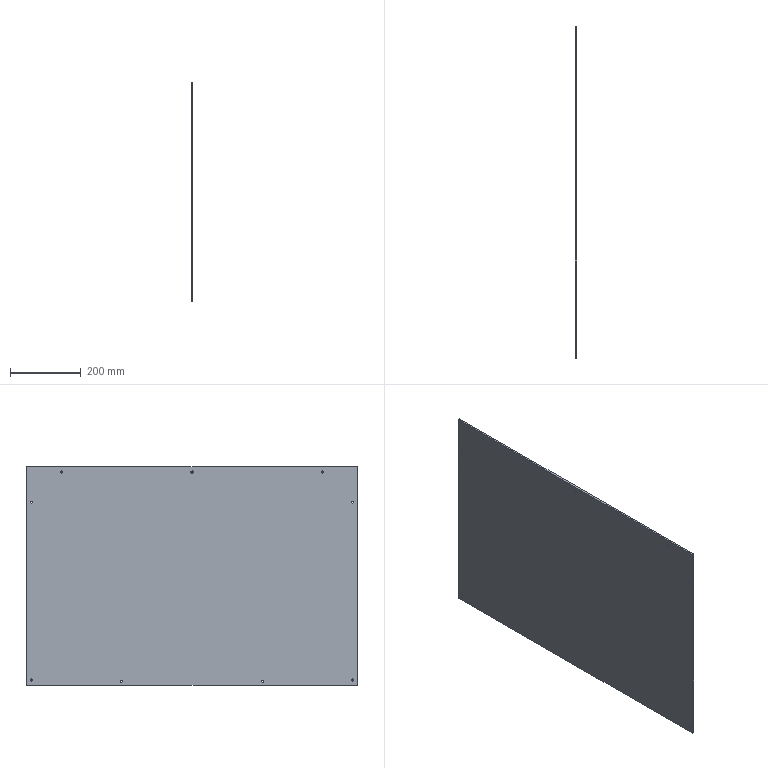Part | SolidWorks | features Chamfer 1, Extrusion 1, ICE 1 | 1 solid | 28 faces | box 5 x 938 x 618 mm | volume 2897138 mm3 | cylinder 18 | plane 10 | commonest cylinder face diameters 6 x18
STEP:
#1=CARTESIAN_POINT('',(5.,-200.,-301.));
#2=VERTEX_POINT('',#1);
#3=CARTESIAN_POINT('',(5.,-200.,-295.));
#4=VERTEX_POINT('',#3);
#5=CARTESIAN_POINT('',(5.,-200.,-298.));
#6=DIRECTION('',(-1.,0.,0.));
#7=DIRECTION('',(0.,0.,1.));
#8=AXIS2_PLACEMENT_3D('',#5,#6,#7);
#9=CIRCLE('',#8,3.);
#10=EDGE_CURVE('',#2,#4,#9,.T.);
#11=ORIENTED_EDGE('',*,*,#10,.F.);
#12=CARTESIAN_POINT('',(0.,-200.,-301.));
#13=VERTEX_POINT('',#12);
#14=CARTESIAN_POINT('',(5.,-200.,-301.));
#15=DIRECTION('',(-1.,0.,0.));
#16=VECTOR('',#15,1000.);
#17=LINE('',#14,#16);
#18=EDGE_CURVE('',#2,#13,#17,.T.);
#19=ORIENTED_EDGE('',*,*,#18,.T.);
#20=CARTESIAN_POINT('',(0.,-200.,-295.));
#21=VERTEX_POINT('',#20);
#22=CARTESIAN_POINT('',(0.,-200.,-298.));
#23=DIRECTION('',(-1.,0.,0.));
#24=DIRECTION('',(0.,0.,1.));
#25=AXIS2_PLACEMENT_3D('',#22,#23,#24);
#26=CIRCLE('',#25,3.);
#27=EDGE_CURVE('',#13,#21,#26,.T.);
#28=ORIENTED_EDGE('',*,*,#27,.T.);
#29=CARTESIAN_POINT('',(5.,-200.,-295.));
#30=DIRECTION('',(-1.,0.,0.));
#31=VECTOR('',#30,1000.);
#32=LINE('',#29,#31);
#33=EDGE_CURVE('',#4,#21,#32,.T.);
#34=ORIENTED_EDGE('',*,*,#33,.F.);
#35=EDGE_LOOP('',(#11,#19,#28,#34));
#36=FACE_OUTER_BOUND('',#35,.T.);
#37=CARTESIAN_POINT('',(5.,-200.,-298.));
#38=DIRECTION('',(-1.,0.,0.));
#39=DIRECTION('',(0.,0.,1.));
#40=AXIS2_PLACEMENT_3D('',#37,#38,#39);
#41=CYLINDRICAL_SURFACE('',#40,3.);
#42=ADVANCED_FACE('',(#36),#41,.F.);
#43=CARTESIAN_POINT('',(5.,200.,-301.));
#44=VERTEX_POINT('',#43);
#45=CARTESIAN_POINT('',(5.,200.,-295.));
#46=VERTEX_POINT('',#45);
#47=CARTESIAN_POINT('',(5.,200.,-298.));
#48=DIRECTION('',(-1.,0.,0.));
#49=DIRECTION('',(0.,0.,1.));
#50=AXIS2_PLACEMENT_3D('',#47,#48,#49);
#51=CIRCLE('',#50,3.);
#52=EDGE_CURVE('',#44,#46,#51,.T.);
#53=ORIENTED_EDGE('',*,*,#52,.F.);
#54=CARTESIAN_POINT('',(0.,200.,-301.));
#55=VERTEX_POINT('',#54);
#56=CARTESIAN_POINT('',(5.,200.,-301.));
#57=DIRECTION('',(-1.,0.,0.));
#58=VECTOR('',#57,1000.);
#59=LINE('',#56,#58);
#60=EDGE_CURVE('',#44,#55,#59,.T.);
#61=ORIENTED_EDGE('',*,*,#60,.T.);
#62=CARTESIAN_POINT('',(0.,200.,-295.));
#63=VERTEX_POINT('',#62);
#64=CARTESIAN_POINT('',(0.,200.,-298.));
#65=DIRECTION('',(-1.,0.,0.));
#66=DIRECTION('',(0.,0.,1.));
#67=AXIS2_PLACEMENT_3D('',#64,#65,#66);
#68=CIRCLE('',#67,3.);
#69=EDGE_CURVE('',#55,#63,#68,.T.);
#70=ORIENTED_EDGE('',*,*,#69,.T.);
#71=CARTESIAN_POINT('',(5.,200.,-295.));
#72=DIRECTION('',(-1.,0.,0.));
#73=VECTOR('',#72,1000.);
#74=LINE('',#71,#73);
#75=EDGE_CURVE('',#46,#63,#74,.T.);
#76=ORIENTED_EDGE('',*,*,#75,.F.);
#77=EDGE_LOOP('',(#53,#61,#70,#76));
#78=FACE_OUTER_BOUND('',#77,.T.);
#79=CARTESIAN_POINT('',(5.,200.,-298.));
#80=DIRECTION('',(-1.,0.,0.));
#81=DIRECTION('',(0.,0.,1.));
#82=AXIS2_PLACEMENT_3D('',#79,#80,#81);
#83=CYLINDRICAL_SURFACE('',#82,3.);
#84=ADVANCED_FACE('',(#78),#83,.F.);
#85=CARTESIAN_POINT('',(5.,0.,291.));
#86=VERTEX_POINT('',#85);
#87=CARTESIAN_POINT('',(5.,0.,297.));
#88=VERTEX_POINT('',#87);
#89=CARTESIAN_POINT('',(5.,0.,294.));
#90=DIRECTION('',(-1.,0.,0.));
#91=DIRECTION('',(0.,0.,1.));
#92=AXIS2_PLACEMENT_3D('',#89,#90,#91);
#93=CIRCLE('',#92,3.);
#94=EDGE_CURVE('',#86,#88,#93,.T.);
#95=ORIENTED_EDGE('',*,*,#94,.F.);
#96=CARTESIAN_POINT('',(0.,0.,291.));
#97=VERTEX_POINT('',#96);
#98=CARTESIAN_POINT('',(5.,0.,291.));
#99=DIRECTION('',(-1.,0.,0.));
#100=VECTOR('',#99,1000.);
#101=LINE('',#98,#100);
#102=EDGE_CURVE('',#86,#97,#101,.T.);
#103=ORIENTED_EDGE('',*,*,#102,.T.);
#104=CARTESIAN_POINT('',(0.,0.,297.));
#105=VERTEX_POINT('',#104);
#106=CARTESIAN_POINT('',(0.,0.,294.));
#107=DIRECTION('',(-1.,0.,0.));
#108=DIRECTION('',(0.,0.,1.));
#109=AXIS2_PLACEMENT_3D('',#106,#107,#108);
#110=CIRCLE('',#109,3.);
#111=EDGE_CURVE('',#97,#105,#110,.T.);
#112=ORIENTED_EDGE('',*,*,#111,.T.);
#113=CARTESIAN_POINT('',(5.,0.,297.));
#114=DIRECTION('',(-1.,0.,0.));
#115=VECTOR('',#114,1000.);
#116=LINE('',#113,#115);
#117=EDGE_CURVE('',#88,#105,#116,.T.);
#118=ORIENTED_EDGE('',*,*,#117,.F.);
#119=EDGE_LOOP('',(#95,#103,#112,#118));
#120=FACE_OUTER_BOUND('',#119,.T.);
#121=CARTESIAN_POINT('',(5.,0.,294.));
#122=DIRECTION('',(-1.,0.,0.));
#123=DIRECTION('',(0.,0.,1.));
#124=AXIS2_PLACEMENT_3D('',#121,#122,#123);
#125=CYLINDRICAL_SURFACE('',#124,3.);
#126=ADVANCED_FACE('',(#120),#125,.F.);
#127=CARTESIAN_POINT('',(5.,-454.,206.));
#128=VERTEX_POINT('',#127);
#129=CARTESIAN_POINT('',(5.,-454.,212.));
#130=VERTEX_POINT('',#129);
#131=CARTESIAN_POINT('',(5.,-454.,209.));
#132=DIRECTION('',(-1.,0.,0.));
#133=DIRECTION('',(0.,0.,1.));
#134=AXIS2_PLACEMENT_3D('',#131,#132,#133);
#135=CIRCLE('',#134,3.);
#136=EDGE_CURVE('',#128,#130,#135,.T.);
#137=ORIENTED_EDGE('',*,*,#136,.F.);
#138=CARTESIAN_POINT('',(0.,-454.,206.));
#139=VERTEX_POINT('',#138);
#140=CARTESIAN_POINT('',(5.,-454.,206.));
#141=DIRECTION('',(-1.,0.,0.));
#142=VECTOR('',#141,1000.);
#143=LINE('',#140,#142);
#144=EDGE_CURVE('',#128,#139,#143,.T.);
#145=ORIENTED_EDGE('',*,*,#144,.T.);
#146=CARTESIAN_POINT('',(0.,-454.,212.));
#147=VERTEX_POINT('',#146);
#148=CARTESIAN_POINT('',(0.,-454.,209.));
#149=DIRECTION('',(-1.,0.,0.));
#150=DIRECTION('',(0.,0.,1.));
#151=AXIS2_PLACEMENT_3D('',#148,#149,#150);
#152=CIRCLE('',#151,3.);
#153=EDGE_CURVE('',#139,#147,#152,.T.);
#154=ORIENTED_EDGE('',*,*,#153,.T.);
#155=CARTESIAN_POINT('',(5.,-454.,212.));
#156=DIRECTION('',(-1.,0.,0.));
#157=VECTOR('',#156,1000.);
#158=LINE('',#155,#157);
#159=EDGE_CURVE('',#130,#147,#158,.T.);
#160=ORIENTED_EDGE('',*,*,#159,.F.);
#161=EDGE_LOOP('',(#137,#145,#154,#160));
#162=FACE_OUTER_BOUND('',#161,.T.);
#163=CARTESIAN_POINT('',(5.,-454.,209.));
#164=DIRECTION('',(-1.,0.,0.));
#165=DIRECTION('',(0.,0.,1.));
#166=AXIS2_PLACEMENT_3D('',#163,#164,#165);
#167=CYLINDRICAL_SURFACE('',#166,3.);
#168=ADVANCED_FACE('',(#162),#167,.F.);
#169=CARTESIAN_POINT('',(5.,-369.,291.));
#170=VERTEX_POINT('',#169);
#171=CARTESIAN_POINT('',(5.,-369.,297.));
#172=VERTEX_POINT('',#171);
#173=CARTESIAN_POINT('',(5.,-369.,294.));
#174=DIRECTION('',(-1.,0.,0.));
#175=DIRECTION('',(0.,0.,1.));
#176=AXIS2_PLACEMENT_3D('',#173,#174,#175);
#177=CIRCLE('',#176,3.);
#178=EDGE_CURVE('',#170,#172,#177,.T.);
#179=ORIENTED_EDGE('',*,*,#178,.F.);
#180=CARTESIAN_POINT('',(0.,-369.,291.));
#181=VERTEX_POINT('',#180);
#182=CARTESIAN_POINT('',(5.,-369.,291.));
#183=DIRECTION('',(-1.,0.,0.));
#184=VECTOR('',#183,1000.);
#185=LINE('',#182,#184);
#186=EDGE_CURVE('',#170,#181,#185,.T.);
#187=ORIENTED_EDGE('',*,*,#186,.T.);
#188=CARTESIAN_POINT('',(0.,-369.,297.));
#189=VERTEX_POINT('',#188);
#190=CARTESIAN_POINT('',(0.,-369.,294.));
#191=DIRECTION('',(-1.,0.,0.));
#192=DIRECTION('',(0.,0.,1.));
#193=AXIS2_PLACEMENT_3D('',#190,#191,#192);
#194=CIRCLE('',#193,3.);
#195=EDGE_CURVE('',#181,#189,#194,.T.);
#196=ORIENTED_EDGE('',*,*,#195,.T.);
#197=CARTESIAN_POINT('',(5.,-369.,297.));
#198=DIRECTION('',(-1.,0.,0.));
#199=VECTOR('',#198,1000.);
#200=LINE('',#197,#199);
#201=EDGE_CURVE('',#172,#189,#200,.T.);
#202=ORIENTED_EDGE('',*,*,#201,.F.);
#203=EDGE_LOOP('',(#179,#187,#196,#202));
#204=FACE_OUTER_BOUND('',#203,.T.);
#205=CARTESIAN_POINT('',(5.,-369.,294.));
#206=DIRECTION('',(-1.,0.,0.));
#207=DIRECTION('',(0.,0.,1.));
#208=AXIS2_PLACEMENT_3D('',#205,#206,#207);
#209=CYLINDRICAL_SURFACE('',#208,3.);
#210=ADVANCED_FACE('',(#204),#209,.F.);
#211=CARTESIAN_POINT('',(5.,369.,291.));
#212=VERTEX_POINT('',#211);
#213=CARTESIAN_POINT('',(5.,369.,297.));
#214=VERTEX_POINT('',#213);
#215=CARTESIAN_POINT('',(5.,369.,294.));
#216=DIRECTION('',(-1.,0.,0.));
#217=DIRECTION('',(0.,0.,1.));
#218=AXIS2_PLACEMENT_3D('',#215,#216,#217);
#219=CIRCLE('',#218,3.);
#220=EDGE_CURVE('',#212,#214,#219,.T.);
#221=ORIENTED_EDGE('',*,*,#220,.F.);
#222=CARTESIAN_POINT('',(0.,369.,291.));
#223=VERTEX_POINT('',#222);
#224=CARTESIAN_POINT('',(5.,369.,291.));
#225=DIRECTION('',(-1.,0.,0.));
#226=VECTOR('',#225,1000.);
#227=LINE('',#224,#226);
#228=EDGE_CURVE('',#212,#223,#227,.T.);
#229=ORIENTED_EDGE('',*,*,#228,.T.);
#230=CARTESIAN_POINT('',(0.,369.,297.));
#231=VERTEX_POINT('',#230);
#232=CARTESIAN_POINT('',(0.,369.,294.));
#233=DIRECTION('',(-1.,0.,0.));
#234=DIRECTION('',(0.,0.,1.));
#235=AXIS2_PLACEMENT_3D('',#232,#233,#234);
#236=CIRCLE('',#235,3.);
#237=EDGE_CURVE('',#223,#231,#236,.T.);
#238=ORIENTED_EDGE('',*,*,#237,.T.);
#239=CARTESIAN_POINT('',(5.,369.,297.));
#240=DIRECTION('',(-1.,0.,0.));
#241=VECTOR('',#240,1000.);
#242=LINE('',#239,#241);
#243=EDGE_CURVE('',#214,#231,#242,.T.);
#244=ORIENTED_EDGE('',*,*,#243,.F.);
#245=EDGE_LOOP('',(#221,#229,#238,#244));
#246=FACE_OUTER_BOUND('',#245,.T.);
#247=CARTESIAN_POINT('',(5.,369.,294.));
#248=DIRECTION('',(-1.,0.,0.));
#249=DIRECTION('',(0.,0.,1.));
#250=AXIS2_PLACEMENT_3D('',#247,#248,#249);
#251=CYLINDRICAL_SURFACE('',#250,3.);
#252=ADVANCED_FACE('',(#246),#251,.F.);
#253=CARTESIAN_POINT('',(5.,454.,206.));
#254=VERTEX_POINT('',#253);
#255=CARTESIAN_POINT('',(5.,454.,212.));
#256=VERTEX_POINT('',#255);
#257=CARTESIAN_POINT('',(5.,454.,209.));
#258=DIRECTION('',(-1.,0.,0.));
#259=DIRECTION('',(0.,0.,1.));
#260=AXIS2_PLACEMENT_3D('',#257,#258,#259);
#261=CIRCLE('',#260,3.);
#262=EDGE_CURVE('',#254,#256,#261,.T.);
#263=ORIENTED_EDGE('',*,*,#262,.F.);
#264=CARTESIAN_POINT('',(0.,454.,206.));
#265=VERTEX_POINT('',#264);
#266=CARTESIAN_POINT('',(5.,454.,206.));
#267=DIRECTION('',(-1.,0.,0.));
#268=VECTOR('',#267,1000.);
#269=LINE('',#266,#268);
#270=EDGE_CURVE('',#254,#265,#269,.T.);
#271=ORIENTED_EDGE('',*,*,#270,.T.);
#272=CARTESIAN_POINT('',(0.,454.,212.));
#273=VERTEX_POINT('',#272);
#274=CARTESIAN_POINT('',(0.,454.,209.));
#275=DIRECTION('',(-1.,0.,0.));
#276=DIRECTION('',(0.,0.,1.));
#277=AXIS2_PLACEMENT_3D('',#274,#275,#276);
#278=CIRCLE('',#277,3.);
#279=EDGE_CURVE('',#265,#273,#278,.T.);
#280=ORIENTED_EDGE('',*,*,#279,.T.);
#281=CARTESIAN_POINT('',(5.,454.,212.));
#282=DIRECTION('',(-1.,0.,0.));
#283=VECTOR('',#282,1000.);
#284=LINE('',#281,#283);
#285=EDGE_CURVE('',#256,#273,#284,.T.);
#286=ORIENTED_EDGE('',*,*,#285,.F.);
#287=EDGE_LOOP('',(#263,#271,#280,#286));
#288=FACE_OUTER_BOUND('',#287,.T.);
#289=CARTESIAN_POINT('',(5.,454.,209.));
#290=DIRECTION('',(-1.,0.,0.));
#291=DIRECTION('',(0.,0.,1.));
#292=AXIS2_PLACEMENT_3D('',#289,#290,#291);
#293=CYLINDRICAL_SURFACE('',#292,3.);
#294=ADVANCED_FACE('',(#288),#293,.F.);
#295=CARTESIAN_POINT('',(5.,-454.,-297.));
#296=VERTEX_POINT('',#295);
#297=CARTESIAN_POINT('',(5.,-454.,-291.));
#298=VERTEX_POINT('',#297);
#299=CARTESIAN_POINT('',(5.,-454.,-294.));
#300=DIRECTION('',(-1.,0.,0.));
#301=DIRECTION('',(0.,0.,-1.));
#302=AXIS2_PLACEMENT_3D('',#299,#300,#301);
#303=CIRCLE('',#302,3.);
#304=EDGE_CURVE('',#296,#298,#303,.T.);
#305=ORIENTED_EDGE('',*,*,#304,.F.);
#306=CARTESIAN_POINT('',(0.,-454.,-297.));
#307=VERTEX_POINT('',#306);
#308=CARTESIAN_POINT('',(5.,-454.,-297.));
#309=DIRECTION('',(-1.,0.,0.));
#310=VECTOR('',#309,1000.);
#311=LINE('',#308,#310);
#312=EDGE_CURVE('',#296,#307,#311,.T.);
#313=ORIENTED_EDGE('',*,*,#312,.T.);
#314=CARTESIAN_POINT('',(0.,-454.,-291.));
#315=VERTEX_POINT('',#314);
#316=CARTESIAN_POINT('',(0.,-454.,-294.));
#317=DIRECTION('',(-1.,0.,0.));
#318=DIRECTION('',(0.,0.,-1.));
#319=AXIS2_PLACEMENT_3D('',#316,#317,#318);
#320=CIRCLE('',#319,3.);
#321=EDGE_CURVE('',#307,#315,#320,.T.);
#322=ORIENTED_EDGE('',*,*,#321,.T.);
#323=CARTESIAN_POINT('',(5.,-454.,-291.));
#324=DIRECTION('',(-1.,0.,0.));
#325=VECTOR('',#324,1000.);
#326=LINE('',#323,#325);
#327=EDGE_CURVE('',#298,#315,#326,.T.);
#328=ORIENTED_EDGE('',*,*,#327,.F.);
#329=EDGE_LOOP('',(#305,#313,#322,#328));
#330=FACE_OUTER_BOUND('',#329,.T.);
#331=CARTESIAN_POINT('',(5.,-454.,-294.));
#332=DIRECTION('',(-1.,0.,0.));
#333=DIRECTION('',(0.,0.,1.));
#334=AXIS2_PLACEMENT_3D('',#331,#332,#333);
#335=CYLINDRICAL_SURFACE('',#334,3.);
#336=ADVANCED_FACE('',(#330),#335,.F.);
#337=CARTESIAN_POINT('',(5.,454.,-297.));
#338=VERTEX_POINT('',#337);
#339=CARTESIAN_POINT('',(5.,454.,-291.));
#340=VERTEX_POINT('',#339);
#341=CARTESIAN_POINT('',(5.,454.,-294.));
#342=DIRECTION('',(-1.,0.,0.));
#343=DIRECTION('',(0.,0.,1.));
#344=AXIS2_PLACEMENT_3D('',#341,#342,#343);
#345=CIRCLE('',#344,3.);
#346=EDGE_CURVE('',#338,#340,#345,.T.);
#347=ORIENTED_EDGE('',*,*,#346,.F.);
#348=CARTESIAN_POINT('',(0.,454.,-297.));
#349=VERTEX_POINT('',#348);
#350=CARTESIAN_POINT('',(5.,454.,-297.));
#351=DIRECTION('',(-1.,0.,0.));
#352=VECTOR('',#351,1000.);
#353=LINE('',#350,#352);
#354=EDGE_CURVE('',#338,#349,#353,.T.);
#355=ORIENTED_EDGE('',*,*,#354,.T.);
#356=CARTESIAN_POINT('',(0.,454.,-291.));
#357=VERTEX_POINT('',#356);
#358=CARTESIAN_POINT('',(0.,454.,-294.));
#359=DIRECTION('',(-1.,0.,0.));
#360=DIRECTION('',(0.,0.,1.));
#361=AXIS2_PLACEMENT_3D('',#358,#359,#360);
#362=CIRCLE('',#361,3.);
#363=EDGE_CURVE('',#349,#357,#362,.T.);
#364=ORIENTED_EDGE('',*,*,#363,.T.);
#365=CARTESIAN_POINT('',(5.,454.,-291.));
#366=DIRECTION('',(-1.,0.,0.));
#367=VECTOR('',#366,1000.);
#368=LINE('',#365,#367);
#369=EDGE_CURVE('',#340,#357,#368,.T.);
#370=ORIENTED_EDGE('',*,*,#369,.F.);
#371=EDGE_LOOP('',(#347,#355,#364,#370));
#372=FACE_OUTER_BOUND('',#371,.T.);
#373=CARTESIAN_POINT('',(5.,454.,-294.));
#374=DIRECTION('',(-1.,0.,0.));
#375=DIRECTION('',(0.,0.,1.));
#376=AXIS2_PLACEMENT_3D('',#373,#374,#375);
#377=CYLINDRICAL_SURFACE('',#376,3.);
#378=ADVANCED_FACE('',(#372),#377,.F.);
#379=CARTESIAN_POINT('',(0.,468.,309.));
#380=VERTEX_POINT('',#379);
#381=CARTESIAN_POINT('',(0.,-468.,309.));
#382=VERTEX_POINT('',#381);
#383=CARTESIAN_POINT('',(0.,469.,309.));
#384=DIRECTION('',(0.,-1.,0.));
#385=VECTOR('',#384,1000.);
#386=LINE('',#383,#385);
#387=EDGE_CURVE('',#380,#382,#386,.T.);
#388=ORIENTED_EDGE('',*,*,#387,.T.);
#389=CARTESIAN_POINT('',(5.,-468.,309.));
#390=VERTEX_POINT('',#389);
#391=CARTESIAN_POINT('',(5.,-468.,309.));
#392=DIRECTION('',(1.,0.,0.));
#393=VECTOR('',#392,1000.);
#394=LINE('',#391,#393);
#395=EDGE_CURVE('',#382,#390,#394,.T.);
#396=ORIENTED_EDGE('',*,*,#395,.T.);
#397=CARTESIAN_POINT('',(5.,468.,309.));
#398=VERTEX_POINT('',#397);
#399=CARTESIAN_POINT('',(5.,469.,309.));
#400=DIRECTION('',(0.,-1.,0.));
#401=VECTOR('',#400,1000.);
#402=LINE('',#399,#401);
#403=EDGE_CURVE('',#398,#390,#402,.T.);
#404=ORIENTED_EDGE('',*,*,#403,.F.);
#405=CARTESIAN_POINT('',(5.,468.,309.));
#406=DIRECTION('',(-1.,0.,0.));
#407=VECTOR('',#406,1000.);
#408=LINE('',#405,#407);
#409=EDGE_CURVE('',#398,#380,#408,.T.);
#410=ORIENTED_EDGE('',*,*,#409,.T.);
#411=EDGE_LOOP('',(#388,#396,#404,#410));
#412=FACE_OUTER_BOUND('',#411,.T.);
#413=CARTESIAN_POINT('',(5.,469.,309.));
#414=DIRECTION('',(0.,0.,-1.));
#415=DIRECTION('',(0.,1.,0.));
#416=AXIS2_PLACEMENT_3D('',#413,#414,#415);
#417=PLANE('',#416);
#418=ADVANCED_FACE('',(#412),#417,.F.);
#419=CARTESIAN_POINT('',(0.,-469.,308.));
#420=VERTEX_POINT('',#419);
#421=CARTESIAN_POINT('',(0.,-469.,-308.));
#422=VERTEX_POINT('',#421);
#423=CARTESIAN_POINT('',(0.,-469.,-309.));
#424=DIRECTION('',(0.,0.,-1.));
#425=VECTOR('',#424,1000.);
#426=LINE('',#423,#425);
#427=EDGE_CURVE('',#420,#422,#426,.T.);
#428=ORIENTED_EDGE('',*,*,#427,.T.);
#429=CARTESIAN_POINT('',(5.,-469.,-308.));
#430=VERTEX_POINT('',#429);
#431=CARTESIAN_POINT('',(5.,-469.,-308.));
#432=DIRECTION('',(1.,0.,0.));
#433=VECTOR('',#432,1000.);
#434=LINE('',#431,#433);
#435=EDGE_CURVE('',#422,#430,#434,.T.);
#436=ORIENTED_EDGE('',*,*,#435,.T.);
#437=CARTESIAN_POINT('',(5.,-469.,308.));
#438=VERTEX_POINT('',#437);
#439=CARTESIAN_POINT('',(5.,-469.,-309.));
#440=DIRECTION('',(0.,0.,-1.));
#441=VECTOR('',#440,1000.);
#442=LINE('',#439,#441);
#443=EDGE_CURVE('',#438,#430,#442,.T.);
#444=ORIENTED_EDGE('',*,*,#443,.F.);
#445=CARTESIAN_POINT('',(5.,-469.,308.));
#446=DIRECTION('',(-1.,0.,0.));
#447=VECTOR('',#446,1000.);
#448=LINE('',#445,#447);
#449=EDGE_CURVE('',#438,#420,#448,.T.);
#450=ORIENTED_EDGE('',*,*,#449,.T.);
#451=EDGE_LOOP('',(#428,#436,#444,#450));
#452=FACE_OUTER_BOUND('',#451,.T.);
#453=CARTESIAN_POINT('',(5.,-469.,-309.));
#454=DIRECTION('',(0.,1.,0.));
#455=DIRECTION('',(0.,0.,1.));
#456=AXIS2_PLACEMENT_3D('',#453,#454,#455);
#457=PLANE('',#456);
#458=ADVANCED_FACE('',(#452),#457,.F.);
#459=CARTESIAN_POINT('',(5.,-468.,-309.));
#460=VERTEX_POINT('',#459);
#461=CARTESIAN_POINT('',(5.,468.,-309.));
#462=VERTEX_POINT('',#461);
#463=CARTESIAN_POINT('',(5.,469.,-309.));
#464=DIRECTION('',(0.,1.,0.));
#465=VECTOR('',#464,1000.);
#466=LINE('',#463,#465);
#467=EDGE_CURVE('',#460,#462,#466,.T.);
#468=ORIENTED_EDGE('',*,*,#467,.F.);
#469=CARTESIAN_POINT('',(0.,-468.,-309.));
#470=VERTEX_POINT('',#469);
#471=CARTESIAN_POINT('',(5.,-468.,-309.));
#472=DIRECTION('',(-1.,0.,0.));
#473=VECTOR('',#472,1000.);
#474=LINE('',#471,#473);
#475=EDGE_CURVE('',#460,#470,#474,.T.);
#476=ORIENTED_EDGE('',*,*,#475,.T.);
#477=CARTESIAN_POINT('',(0.,468.,-309.));
#478=VERTEX_POINT('',#477);
#479=CARTESIAN_POINT('',(0.,469.,-309.));
#480=DIRECTION('',(0.,1.,0.));
#481=VECTOR('',#480,1000.);
#482=LINE('',#479,#481);
#483=EDGE_CURVE('',#470,#478,#482,.T.);
#484=ORIENTED_EDGE('',*,*,#483,.T.);
#485=CARTESIAN_POINT('',(5.,468.,-309.));
#486=DIRECTION('',(1.,0.,0.));
#487=VECTOR('',#486,1000.);
#488=LINE('',#485,#487);
#489=EDGE_CURVE('',#478,#462,#488,.T.);
#490=ORIENTED_EDGE('',*,*,#489,.T.);
#491=EDGE_LOOP('',(#468,#476,#484,#490));
#492=FACE_OUTER_BOUND('',#491,.T.);
#493=CARTESIAN_POINT('',(5.,469.,-309.));
#494=DIRECTION('',(0.,0.,1.));
#495=DIRECTION('',(0.,-1.,0.));
#496=AXIS2_PLACEMENT_3D('',#493,#494,#495);
#497=PLANE('',#496);
#498=ADVANCED_FACE('',(#492),#497,.F.);
#499=CARTESIAN_POINT('',(5.,469.,-308.));
#500=VERTEX_POINT('',#499);
#501=CARTESIAN_POINT('',(5.,469.,308.));
#502=VERTEX_POINT('',#501);
#503=CARTESIAN_POINT('',(5.,469.,-309.));
#504=DIRECTION('',(0.,0.,1.));
#505=VECTOR('',#504,1000.);
#506=LINE('',#503,#505);
#507=EDGE_CURVE('',#500,#502,#506,.T.);
#508=ORIENTED_EDGE('',*,*,#507,.F.);
#509=CARTESIAN_POINT('',(0.,469.,-308.));
#510=VERTEX_POINT('',#509);
#511=CARTESIAN_POINT('',(5.,469.,-308.));
#512=DIRECTION('',(-1.,0.,0.));
#513=VECTOR('',#512,1000.);
#514=LINE('',#511,#513);
#515=EDGE_CURVE('',#500,#510,#514,.T.);
#516=ORIENTED_EDGE('',*,*,#515,.T.);
#517=CARTESIAN_POINT('',(0.,469.,308.));
#518=VERTEX_POINT('',#517);
#519=CARTESIAN_POINT('',(0.,469.,-309.));
#520=DIRECTION('',(0.,0.,1.));
#521=VECTOR('',#520,1000.);
#522=LINE('',#519,#521);
#523=EDGE_CURVE('',#510,#518,#522,.T.);
#524=ORIENTED_EDGE('',*,*,#523,.T.);
#525=CARTESIAN_POINT('',(5.,469.,308.));
#526=DIRECTION('',(1.,0.,0.));
#527=VECTOR('',#526,1000.);
#528=LINE('',#525,#527);
#529=EDGE_CURVE('',#518,#502,#528,.T.);
#530=ORIENTED_EDGE('',*,*,#529,.T.);
#531=EDGE_LOOP('',(#508,#516,#524,#530));
#532=FACE_OUTER_BOUND('',#531,.T.);
#533=CARTESIAN_POINT('',(5.,469.,-309.));
#534=DIRECTION('',(0.,-1.,0.));
#535=DIRECTION('',(0.,0.,-1.));
#536=AXIS2_PLACEMENT_3D('',#533,#534,#535);
#537=PLANE('',#536);
#538=ADVANCED_FACE('',(#532),#537,.F.);
#539=CARTESIAN_POINT('',(5.,-200.,-298.));
#540=DIRECTION('',(-1.,0.,0.));
#541=DIRECTION('',(0.,0.,1.));
#542=AXIS2_PLACEMENT_3D('',#539,#540,#541);
#543=CIRCLE('',#542,3.);
#544=EDGE_CURVE('',#4,#2,#543,.T.);
#545=ORIENTED_EDGE('',*,*,#544,.T.);
#546=ORIENTED_EDGE('',*,*,#10,.T.);
#547=EDGE_LOOP('',(#545,#546));
#548=FACE_BOUND('',#547,.T.);
#549=CARTESIAN_POINT('',(5.,200.,-298.));
#550=DIRECTION('',(-1.,0.,0.));
#551=DIRECTION('',(0.,0.,1.));
#552=AXIS2_PLACEMENT_3D('',#549,#550,#551);
#553=CIRCLE('',#552,3.);
#554=EDGE_CURVE('',#46,#44,#553,.T.);
#555=ORIENTED_EDGE('',*,*,#554,.T.);
#556=ORIENTED_EDGE('',*,*,#52,.T.);
#557=EDGE_LOOP('',(#555,#556));
#558=FACE_BOUND('',#557,.T.);
#559=CARTESIAN_POINT('',(5.,0.,294.));
#560=DIRECTION('',(-1.,0.,0.));
#561=DIRECTION('',(0.,0.,1.));
#562=AXIS2_PLACEMENT_3D('',#559,#560,#561);
#563=CIRCLE('',#562,3.);
#564=EDGE_CURVE('',#88,#86,#563,.T.);
#565=ORIENTED_EDGE('',*,*,#564,.T.);
#566=ORIENTED_EDGE('',*,*,#94,.T.);
#567=EDGE_LOOP('',(#565,#566));
#568=FACE_BOUND('',#567,.T.);
#569=CARTESIAN_POINT('',(5.,-454.,209.));
#570=DIRECTION('',(-1.,0.,0.));
#571=DIRECTION('',(0.,0.,1.));
#572=AXIS2_PLACEMENT_3D('',#569,#570,#571);
#573=CIRCLE('',#572,3.);
#574=EDGE_CURVE('',#130,#128,#573,.T.);
#575=ORIENTED_EDGE('',*,*,#574,.T.);
#576=ORIENTED_EDGE('',*,*,#136,.T.);
#577=EDGE_LOOP('',(#575,#576));
#578=FACE_BOUND('',#577,.T.);
#579=CARTESIAN_POINT('',(5.,-369.,294.));
#580=DIRECTION('',(-1.,0.,0.));
#581=DIRECTION('',(0.,0.,1.));
#582=AXIS2_PLACEMENT_3D('',#579,#580,#581);
#583=CIRCLE('',#582,3.);
#584=EDGE_CURVE('',#172,#170,#583,.T.);
#585=ORIENTED_EDGE('',*,*,#584,.T.);
#586=ORIENTED_EDGE('',*,*,#178,.T.);
#587=EDGE_LOOP('',(#585,#586));
#588=FACE_BOUND('',#587,.T.);
#589=CARTESIAN_POINT('',(5.,369.,294.));
#590=DIRECTION('',(-1.,0.,0.));
#591=DIRECTION('',(0.,0.,1.));
#592=AXIS2_PLACEMENT_3D('',#589,#590,#591);
#593=CIRCLE('',#592,3.);
#594=EDGE_CURVE('',#214,#212,#593,.T.);
#595=ORIENTED_EDGE('',*,*,#594,.T.);
#596=ORIENTED_EDGE('',*,*,#220,.T.);
#597=EDGE_LOOP('',(#595,#596));
#598=FACE_BOUND('',#597,.T.);
#599=CARTESIAN_POINT('',(5.,454.,209.));
#600=DIRECTION('',(-1.,0.,0.));
#601=DIRECTION('',(0.,0.,1.));
#602=AXIS2_PLACEMENT_3D('',#599,#600,#601);
#603=CIRCLE('',#602,3.);
#604=EDGE_CURVE('',#256,#254,#603,.T.);
#605=ORIENTED_EDGE('',*,*,#604,.T.);
#606=ORIENTED_EDGE('',*,*,#262,.T.);
#607=EDGE_LOOP('',(#605,#606));
#608=FACE_BOUND('',#607,.T.);
#609=CARTESIAN_POINT('',(5.,-454.,-294.));
#610=DIRECTION('',(-1.,0.,0.));
#611=DIRECTION('',(0.,0.,-1.));
#612=AXIS2_PLACEMENT_3D('',#609,#610,#611);
#613=CIRCLE('',#612,3.);
#614=EDGE_CURVE('',#298,#296,#613,.T.);
#615=ORIENTED_EDGE('',*,*,#614,.T.);
#616=ORIENTED_EDGE('',*,*,#304,.T.);
#617=EDGE_LOOP('',(#615,#616));
#618=FACE_BOUND('',#617,.T.);
#619=CARTESIAN_POINT('',(5.,454.,-294.));
#620=DIRECTION('',(-1.,0.,0.));
#621=DIRECTION('',(0.,0.,1.));
#622=AXIS2_PLACEMENT_3D('',#619,#620,#621);
#623=CIRCLE('',#622,3.);
#624=EDGE_CURVE('',#340,#338,#623,.T.);
#625=ORIENTED_EDGE('',*,*,#624,.T.);
#626=ORIENTED_EDGE('',*,*,#346,.T.);
#627=EDGE_LOOP('',(#625,#626));
#628=FACE_BOUND('',#627,.T.);
#629=ORIENTED_EDGE('',*,*,#443,.T.);
#630=CARTESIAN_POINT('',(5.,-468.,-309.));
#631=DIRECTION('',(0.,0.7071,-0.7071));
#632=VECTOR('',#631,1000.);
#633=LINE('',#630,#632);
#634=EDGE_CURVE('',#430,#460,#633,.T.);
#635=ORIENTED_EDGE('',*,*,#634,.T.);
#636=ORIENTED_EDGE('',*,*,#467,.T.);
#637=CARTESIAN_POINT('',(5.,469.,-308.));
#638=DIRECTION('',(0.,0.7071,0.7071));
#639=VECTOR('',#638,1000.);
#640=LINE('',#637,#639);
#641=EDGE_CURVE('',#462,#500,#640,.T.);
#642=ORIENTED_EDGE('',*,*,#641,.T.);
#643=ORIENTED_EDGE('',*,*,#507,.T.);
#644=CARTESIAN_POINT('',(5.,468.,309.));
#645=DIRECTION('',(0.,-0.7071,0.7071));
#646=VECTOR('',#645,1000.);
#647=LINE('',#644,#646);
#648=EDGE_CURVE('',#502,#398,#647,.T.);
#649=ORIENTED_EDGE('',*,*,#648,.T.);
#650=ORIENTED_EDGE('',*,*,#403,.T.);
#651=CARTESIAN_POINT('',(5.,-469.,308.));
#652=DIRECTION('',(0.,-0.7071,-0.7071));
#653=VECTOR('',#652,1000.);
#654=LINE('',#651,#653);
#655=EDGE_CURVE('',#390,#438,#654,.T.);
#656=ORIENTED_EDGE('',*,*,#655,.T.);
#657=EDGE_LOOP('',(#629,#635,#636,#642,#643,#649,#650,#656));
#658=FACE_OUTER_BOUND('',#657,.T.);
#659=CARTESIAN_POINT('',(5.,-469.,309.));
#660=DIRECTION('',(-1.,0.,0.));
#661=DIRECTION('',(0.,0.,1.));
#662=AXIS2_PLACEMENT_3D('',#659,#660,#661);
#663=PLANE('',#662);
#664=ADVANCED_FACE('',(#548,#558,#568,#578,#588,#598,#608,#618,#628,#658),#663,.F.);
#665=CARTESIAN_POINT('',(0.,-200.,-298.));
#666=DIRECTION('',(-1.,0.,0.));
#667=DIRECTION('',(0.,0.,1.));
#668=AXIS2_PLACEMENT_3D('',#665,#666,#667);
#669=CIRCLE('',#668,3.);
#670=EDGE_CURVE('',#21,#13,#669,.T.);
#671=ORIENTED_EDGE('',*,*,#670,.F.);
#672=ORIENTED_EDGE('',*,*,#27,.F.);
#673=EDGE_LOOP('',(#671,#672));
#674=FACE_BOUND('',#673,.T.);
#675=CARTESIAN_POINT('',(0.,200.,-298.));
#676=DIRECTION('',(-1.,0.,0.));
#677=DIRECTION('',(0.,0.,1.));
#678=AXIS2_PLACEMENT_3D('',#675,#676,#677);
#679=CIRCLE('',#678,3.);
#680=EDGE_CURVE('',#63,#55,#679,.T.);
#681=ORIENTED_EDGE('',*,*,#680,.F.);
#682=ORIENTED_EDGE('',*,*,#69,.F.);
#683=EDGE_LOOP('',(#681,#682));
#684=FACE_BOUND('',#683,.T.);
#685=CARTESIAN_POINT('',(0.,0.,294.));
#686=DIRECTION('',(-1.,0.,0.));
#687=DIRECTION('',(0.,0.,1.));
#688=AXIS2_PLACEMENT_3D('',#685,#686,#687);
#689=CIRCLE('',#688,3.);
#690=EDGE_CURVE('',#105,#97,#689,.T.);
#691=ORIENTED_EDGE('',*,*,#690,.F.);
#692=ORIENTED_EDGE('',*,*,#111,.F.);
#693=EDGE_LOOP('',(#691,#692));
#694=FACE_BOUND('',#693,.T.);
#695=CARTESIAN_POINT('',(0.,-454.,209.));
#696=DIRECTION('',(-1.,0.,0.));
#697=DIRECTION('',(0.,0.,1.));
#698=AXIS2_PLACEMENT_3D('',#695,#696,#697);
#699=CIRCLE('',#698,3.);
#700=EDGE_CURVE('',#147,#139,#699,.T.);
#701=ORIENTED_EDGE('',*,*,#700,.F.);
#702=ORIENTED_EDGE('',*,*,#153,.F.);
#703=EDGE_LOOP('',(#701,#702));
#704=FACE_BOUND('',#703,.T.);
#705=CARTESIAN_POINT('',(0.,-369.,294.));
#706=DIRECTION('',(-1.,0.,0.));
#707=DIRECTION('',(0.,0.,1.));
#708=AXIS2_PLACEMENT_3D('',#705,#706,#707);
#709=CIRCLE('',#708,3.);
#710=EDGE_CURVE('',#189,#181,#709,.T.);
#711=ORIENTED_EDGE('',*,*,#710,.F.);
#712=ORIENTED_EDGE('',*,*,#195,.F.);
#713=EDGE_LOOP('',(#711,#712));
#714=FACE_BOUND('',#713,.T.);
#715=CARTESIAN_POINT('',(0.,369.,294.));
#716=DIRECTION('',(-1.,0.,0.));
#717=DIRECTION('',(0.,0.,1.));
#718=AXIS2_PLACEMENT_3D('',#715,#716,#717);
#719=CIRCLE('',#718,3.);
#720=EDGE_CURVE('',#231,#223,#719,.T.);
#721=ORIENTED_EDGE('',*,*,#720,.F.);
#722=ORIENTED_EDGE('',*,*,#237,.F.);
#723=EDGE_LOOP('',(#721,#722));
#724=FACE_BOUND('',#723,.T.);
#725=CARTESIAN_POINT('',(0.,454.,209.));
#726=DIRECTION('',(-1.,0.,0.));
#727=DIRECTION('',(0.,0.,1.));
#728=AXIS2_PLACEMENT_3D('',#725,#726,#727);
#729=CIRCLE('',#728,3.);
#730=EDGE_CURVE('',#273,#265,#729,.T.);
#731=ORIENTED_EDGE('',*,*,#730,.F.);
#732=ORIENTED_EDGE('',*,*,#279,.F.);
#733=EDGE_LOOP('',(#731,#732));
#734=FACE_BOUND('',#733,.T.);
#735=CARTESIAN_POINT('',(0.,-454.,-294.));
#736=DIRECTION('',(-1.,0.,0.));
#737=DIRECTION('',(0.,0.,-1.));
#738=AXIS2_PLACEMENT_3D('',#735,#736,#737);
#739=CIRCLE('',#738,3.);
#740=EDGE_CURVE('',#315,#307,#739,.T.);
#741=ORIENTED_EDGE('',*,*,#740,.F.);
#742=ORIENTED_EDGE('',*,*,#321,.F.);
#743=EDGE_LOOP('',(#741,#742));
#744=FACE_BOUND('',#743,.T.);
#745=CARTESIAN_POINT('',(0.,454.,-294.));
#746=DIRECTION('',(-1.,0.,0.));
#747=DIRECTION('',(0.,0.,1.));
#748=AXIS2_PLACEMENT_3D('',#745,#746,#747);
#749=CIRCLE('',#748,3.);
#750=EDGE_CURVE('',#357,#349,#749,.T.);
#751=ORIENTED_EDGE('',*,*,#750,.F.);
#752=ORIENTED_EDGE('',*,*,#363,.F.);
#753=EDGE_LOOP('',(#751,#752));
#754=FACE_BOUND('',#753,.T.);
#755=ORIENTED_EDGE('',*,*,#483,.F.);
#756=CARTESIAN_POINT('',(0.,-777.5,0.5));
#757=DIRECTION('',(0.,-0.7071,0.7071));
#758=VECTOR('',#757,1000.);
#759=LINE('',#756,#758);
#760=EDGE_CURVE('',#470,#422,#759,.T.);
#761=ORIENTED_EDGE('',*,*,#760,.T.);
#762=ORIENTED_EDGE('',*,*,#427,.F.);
#763=CARTESIAN_POINT('',(0.,-468.5,308.5));
#764=DIRECTION('',(0.,0.7071,0.7071));
#765=VECTOR('',#764,1000.);
#766=LINE('',#763,#765);
#767=EDGE_CURVE('',#420,#382,#766,.T.);
#768=ORIENTED_EDGE('',*,*,#767,.T.);
#769=ORIENTED_EDGE('',*,*,#387,.F.);
#770=CARTESIAN_POINT('',(0.,-0.5,777.5));
#771=DIRECTION('',(0.,0.7071,-0.7071));
#772=VECTOR('',#771,1000.);
#773=LINE('',#770,#772);
#774=EDGE_CURVE('',#380,#518,#773,.T.);
#775=ORIENTED_EDGE('',*,*,#774,.T.);
#776=ORIENTED_EDGE('',*,*,#523,.F.);
#777=CARTESIAN_POINT('',(0.,308.5,-468.5));
#778=DIRECTION('',(0.,-0.7071,-0.7071));
#779=VECTOR('',#778,1000.);
#780=LINE('',#777,#779);
#781=EDGE_CURVE('',#510,#478,#780,.T.);
#782=ORIENTED_EDGE('',*,*,#781,.T.);
#783=EDGE_LOOP('',(#755,#761,#762,#768,#769,#775,#776,#782));
#784=FACE_OUTER_BOUND('',#783,.T.);
#785=CARTESIAN_POINT('',(0.,-469.,309.));
#786=DIRECTION('',(-1.,0.,0.));
#787=DIRECTION('',(0.,0.,1.));
#788=AXIS2_PLACEMENT_3D('',#785,#786,#787);
#789=PLANE('',#788);
#790=ADVANCED_FACE('',(#674,#684,#694,#704,#714,#724,#734,#744,#754,#784),#789,.T.);
#791=ORIENTED_EDGE('',*,*,#634,.F.);
#792=ORIENTED_EDGE('',*,*,#435,.F.);
#793=ORIENTED_EDGE('',*,*,#760,.F.);
#794=ORIENTED_EDGE('',*,*,#475,.F.);
#795=EDGE_LOOP('',(#791,#792,#793,#794));
#796=FACE_OUTER_BOUND('',#795,.T.);
#797=CARTESIAN_POINT('',(5.,-468.,-309.));
#798=DIRECTION('',(0.,0.7071,0.7071));
#799=DIRECTION('',(0.,-0.7071,0.7071));
#800=AXIS2_PLACEMENT_3D('',#797,#798,#799);
#801=PLANE('',#800);
#802=ADVANCED_FACE('',(#796),#801,.F.);
#803=ORIENTED_EDGE('',*,*,#655,.F.);
#804=ORIENTED_EDGE('',*,*,#395,.F.);
#805=ORIENTED_EDGE('',*,*,#767,.F.);
#806=ORIENTED_EDGE('',*,*,#449,.F.);
#807=EDGE_LOOP('',(#803,#804,#805,#806));
#808=FACE_OUTER_BOUND('',#807,.T.);
#809=CARTESIAN_POINT('',(5.,-469.,308.));
#810=DIRECTION('',(0.,0.7071,-0.7071));
#811=DIRECTION('',(0.,0.7071,0.7071));
#812=AXIS2_PLACEMENT_3D('',#809,#810,#811);
#813=PLANE('',#812);
#814=ADVANCED_FACE('',(#808),#813,.F.);
#815=ORIENTED_EDGE('',*,*,#641,.F.);
#816=ORIENTED_EDGE('',*,*,#489,.F.);
#817=ORIENTED_EDGE('',*,*,#781,.F.);
#818=ORIENTED_EDGE('',*,*,#515,.F.);
#819=EDGE_LOOP('',(#815,#816,#817,#818));
#820=FACE_OUTER_BOUND('',#819,.T.);
#821=CARTESIAN_POINT('',(5.,469.,-308.));
#822=DIRECTION('',(0.,-0.7071,0.7071));
#823=DIRECTION('',(0.,-0.7071,-0.7071));
#824=AXIS2_PLACEMENT_3D('',#821,#822,#823);
#825=PLANE('',#824);
#826=ADVANCED_FACE('',(#820),#825,.F.);
#827=ORIENTED_EDGE('',*,*,#648,.F.);
#828=ORIENTED_EDGE('',*,*,#529,.F.);
#829=ORIENTED_EDGE('',*,*,#774,.F.);
#830=ORIENTED_EDGE('',*,*,#409,.F.);
#831=EDGE_LOOP('',(#827,#828,#829,#830));
#832=FACE_OUTER_BOUND('',#831,.T.);
#833=CARTESIAN_POINT('',(5.,468.,309.));
#834=DIRECTION('',(0.,-0.7071,-0.7071));
#835=DIRECTION('',(0.,0.7071,-0.7071));
#836=AXIS2_PLACEMENT_3D('',#833,#834,#835);
#837=PLANE('',#836);
#838=ADVANCED_FACE('',(#832),#837,.F.);
#839=ORIENTED_EDGE('',*,*,#354,.F.);
#840=ORIENTED_EDGE('',*,*,#624,.F.);
#841=ORIENTED_EDGE('',*,*,#369,.T.);
#842=ORIENTED_EDGE('',*,*,#750,.T.);
#843=EDGE_LOOP('',(#839,#840,#841,#842));
#844=FACE_OUTER_BOUND('',#843,.T.);
#845=CARTESIAN_POINT('',(5.,454.,-294.));
#846=DIRECTION('',(-1.,0.,0.));
#847=DIRECTION('',(0.,0.,1.));
#848=AXIS2_PLACEMENT_3D('',#845,#846,#847);
#849=CYLINDRICAL_SURFACE('',#848,3.);
#850=ADVANCED_FACE('',(#844),#849,.F.);
#851=ORIENTED_EDGE('',*,*,#312,.F.);
#852=ORIENTED_EDGE('',*,*,#614,.F.);
#853=ORIENTED_EDGE('',*,*,#327,.T.);
#854=ORIENTED_EDGE('',*,*,#740,.T.);
#855=EDGE_LOOP('',(#851,#852,#853,#854));
#856=FACE_OUTER_BOUND('',#855,.T.);
#857=CARTESIAN_POINT('',(5.,-454.,-294.));
#858=DIRECTION('',(-1.,0.,0.));
#859=DIRECTION('',(0.,0.,1.));
#860=AXIS2_PLACEMENT_3D('',#857,#858,#859);
#861=CYLINDRICAL_SURFACE('',#860,3.);
#862=ADVANCED_FACE('',(#856),#861,.F.);
#863=ORIENTED_EDGE('',*,*,#270,.F.);
#864=ORIENTED_EDGE('',*,*,#604,.F.);
#865=ORIENTED_EDGE('',*,*,#285,.T.);
#866=ORIENTED_EDGE('',*,*,#730,.T.);
#867=EDGE_LOOP('',(#863,#864,#865,#866));
#868=FACE_OUTER_BOUND('',#867,.T.);
#869=CARTESIAN_POINT('',(5.,454.,209.));
#870=DIRECTION('',(-1.,0.,0.));
#871=DIRECTION('',(0.,0.,1.));
#872=AXIS2_PLACEMENT_3D('',#869,#870,#871);
#873=CYLINDRICAL_SURFACE('',#872,3.);
#874=ADVANCED_FACE('',(#868),#873,.F.);
#875=ORIENTED_EDGE('',*,*,#228,.F.);
#876=ORIENTED_EDGE('',*,*,#594,.F.);
#877=ORIENTED_EDGE('',*,*,#243,.T.);
#878=ORIENTED_EDGE('',*,*,#720,.T.);
#879=EDGE_LOOP('',(#875,#876,#877,#878));
#880=FACE_OUTER_BOUND('',#879,.T.);
#881=CARTESIAN_POINT('',(5.,369.,294.));
#882=DIRECTION('',(-1.,0.,0.));
#883=DIRECTION('',(0.,0.,1.));
#884=AXIS2_PLACEMENT_3D('',#881,#882,#883);
#885=CYLINDRICAL_SURFACE('',#884,3.);
#886=ADVANCED_FACE('',(#880),#885,.F.);
#887=ORIENTED_EDGE('',*,*,#186,.F.);
#888=ORIENTED_EDGE('',*,*,#584,.F.);
#889=ORIENTED_EDGE('',*,*,#201,.T.);
#890=ORIENTED_EDGE('',*,*,#710,.T.);
#891=EDGE_LOOP('',(#887,#888,#889,#890));
#892=FACE_OUTER_BOUND('',#891,.T.);
#893=CARTESIAN_POINT('',(5.,-369.,294.));
#894=DIRECTION('',(-1.,0.,0.));
#895=DIRECTION('',(0.,0.,1.));
#896=AXIS2_PLACEMENT_3D('',#893,#894,#895);
#897=CYLINDRICAL_SURFACE('',#896,3.);
#898=ADVANCED_FACE('',(#892),#897,.F.);
#899=ORIENTED_EDGE('',*,*,#144,.F.);
#900=ORIENTED_EDGE('',*,*,#574,.F.);
#901=ORIENTED_EDGE('',*,*,#159,.T.);
#902=ORIENTED_EDGE('',*,*,#700,.T.);
#903=EDGE_LOOP('',(#899,#900,#901,#902));
#904=FACE_OUTER_BOUND('',#903,.T.);
#905=CARTESIAN_POINT('',(5.,-454.,209.));
#906=DIRECTION('',(-1.,0.,0.));
#907=DIRECTION('',(0.,0.,1.));
#908=AXIS2_PLACEMENT_3D('',#905,#906,#907);
#909=CYLINDRICAL_SURFACE('',#908,3.);
#910=ADVANCED_FACE('',(#904),#909,.F.);
#911=ORIENTED_EDGE('',*,*,#102,.F.);
#912=ORIENTED_EDGE('',*,*,#564,.F.);
#913=ORIENTED_EDGE('',*,*,#117,.T.);
#914=ORIENTED_EDGE('',*,*,#690,.T.);
#915=EDGE_LOOP('',(#911,#912,#913,#914));
#916=FACE_OUTER_BOUND('',#915,.T.);
#917=CARTESIAN_POINT('',(5.,0.,294.));
#918=DIRECTION('',(-1.,0.,0.));
#919=DIRECTION('',(0.,0.,1.));
#920=AXIS2_PLACEMENT_3D('',#917,#918,#919);
#921=CYLINDRICAL_SURFACE('',#920,3.);
#922=ADVANCED_FACE('',(#916),#921,.F.);
#923=ORIENTED_EDGE('',*,*,#60,.F.);
#924=ORIENTED_EDGE('',*,*,#554,.F.);
#925=ORIENTED_EDGE('',*,*,#75,.T.);
#926=ORIENTED_EDGE('',*,*,#680,.T.);
#927=EDGE_LOOP('',(#923,#924,#925,#926));
#928=FACE_OUTER_BOUND('',#927,.T.);
#929=CARTESIAN_POINT('',(5.,200.,-298.));
#930=DIRECTION('',(-1.,0.,0.));
#931=DIRECTION('',(0.,0.,1.));
#932=AXIS2_PLACEMENT_3D('',#929,#930,#931);
#933=CYLINDRICAL_SURFACE('',#932,3.);
#934=ADVANCED_FACE('',(#928),#933,.F.);
#935=ORIENTED_EDGE('',*,*,#18,.F.);
#936=ORIENTED_EDGE('',*,*,#544,.F.);
#937=ORIENTED_EDGE('',*,*,#33,.T.);
#938=ORIENTED_EDGE('',*,*,#670,.T.);
#939=EDGE_LOOP('',(#935,#936,#937,#938));
#940=FACE_OUTER_BOUND('',#939,.T.);
#941=CARTESIAN_POINT('',(5.,-200.,-298.));
#942=DIRECTION('',(-1.,0.,0.));
#943=DIRECTION('',(0.,0.,1.));
#944=AXIS2_PLACEMENT_3D('',#941,#942,#943);
#945=CYLINDRICAL_SURFACE('',#944,3.);
#946=ADVANCED_FACE('',(#940),#945,.F.);
#947=CLOSED_SHELL('',(#42,#84,#126,#168,#210,#252,#294,#336,#378,#418,#458,#498,#538,#664,#790,#802,#814,#826,#838,#850,#862,#874,#886,#898,#910,#922,#934,#946));
#948=MANIFOLD_SOLID_BREP('',#947);
#949=CARTESIAN_POINT('',(0.,0.,0.));
#950=DIRECTION('',(0.,0.,1.));
#951=DIRECTION('',(1.,0.,0.));
#952=AXIS2_PLACEMENT_3D('',#949,#950,#951);
#953=(LENGTH_UNIT()NAMED_UNIT(*)SI_UNIT(.MILLI.,.METRE.));
#954=UNCERTAINTY_MEASURE_WITH_UNIT(LENGTH_MEASURE(0.00001),#953,'','');
#955=(NAMED_UNIT(*)PLANE_ANGLE_UNIT()SI_UNIT($,.RADIAN.));
#956=(NAMED_UNIT(*)SI_UNIT($,.STERADIAN.)SOLID_ANGLE_UNIT());
#957=(GEOMETRIC_REPRESENTATION_CONTEXT(3)GLOBAL_UNCERTAINTY_ASSIGNED_CONTEXT((#954))GLOBAL_UNIT_ASSIGNED_CONTEXT((#953,#955,#956))REPRESENTATION_CONTEXT('',''));
#958=ADVANCED_BREP_SHAPE_REPRESENTATION('',(#948,#952),#957);